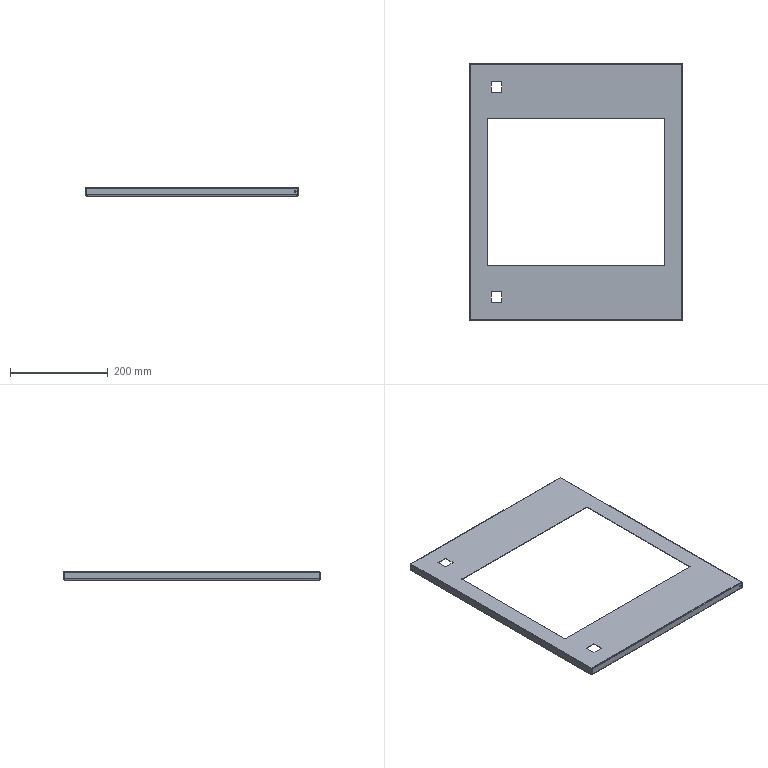Part | STEP file | 1 solid | 110 faces | box 436 x 526 x 17 mm | volume 186343 mm3 | plane 70 | cylinder 28 | spline 12 | commonest cylinder face diameters 2.8 x10 5.2 x6 0.4 x4 2 x4 3 x4